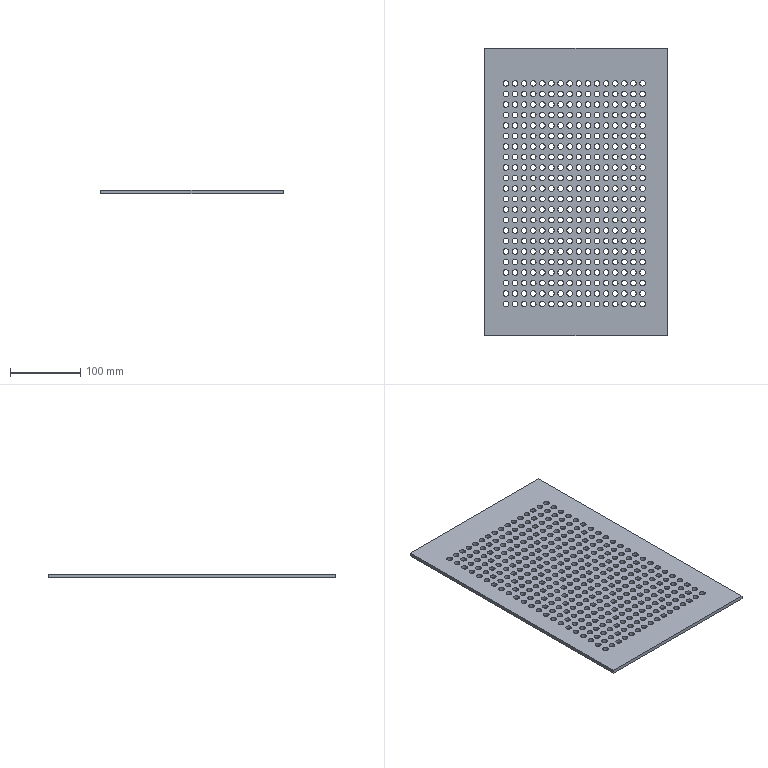Part | STEP file | MYT-A01-P27 | 1 solid | 710 faces | box 260 x 410 x 5 mm | volume 444533 mm3 | cylinder 704 | plane 6 | commonest cylinder face diameters 8 x704